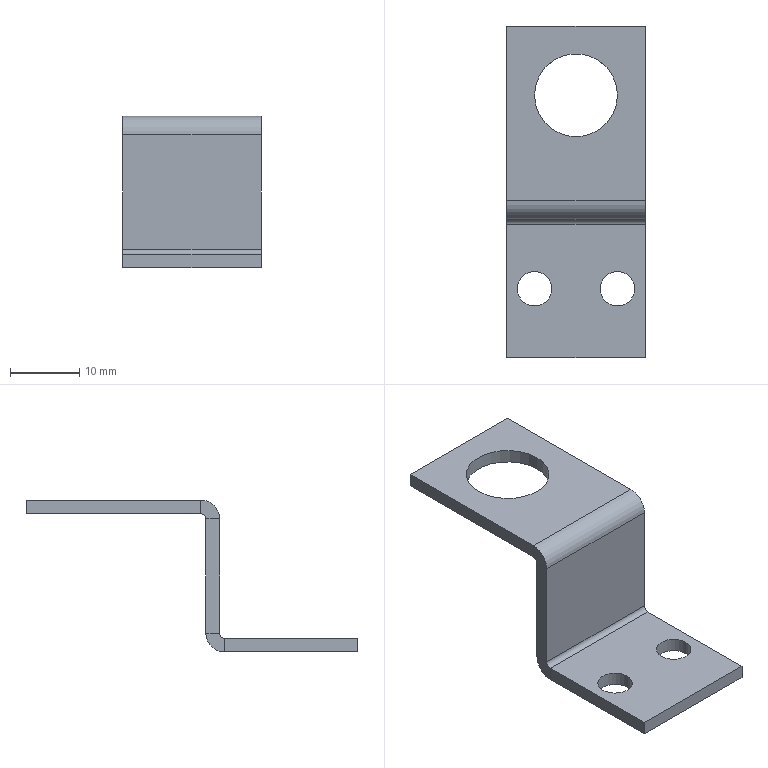Part | STEP file | PN_0011 (proximity switch bracket) | 1 solid | 28 faces | box 20 x 48 x 22 mm | volume 2356 mm3 | plane 18 | cylinder 10 | commonest cylinder face diameters 5 x4 1.473 x2 5.473 x2 12 x2